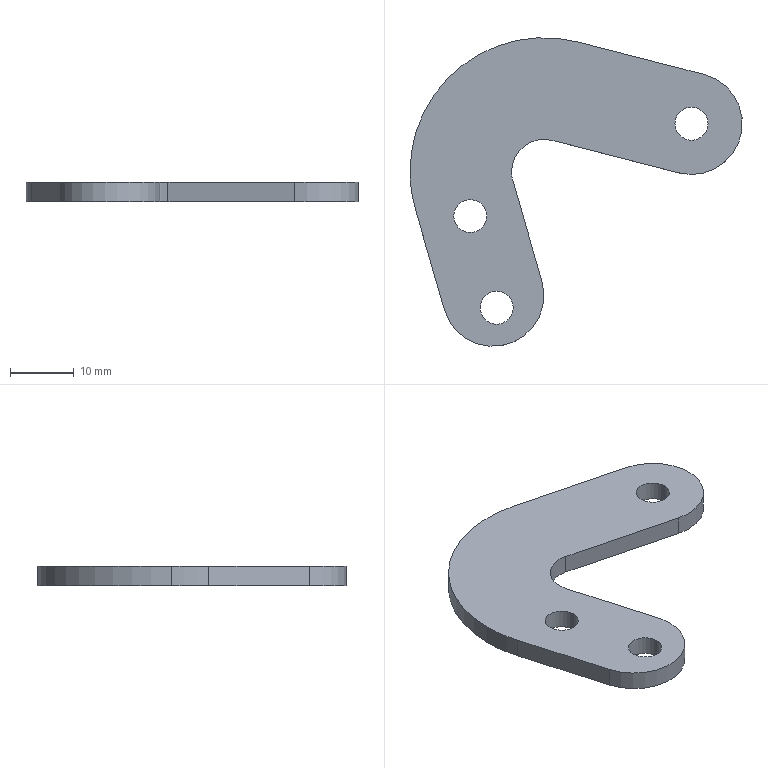Part | SolidWorks | features BaseBody 1 | 1 solid | 18 faces | box 52.312 x 48.572 x 3 mm | volume 3515 mm3 | cylinder 12 | plane 6 | commonest cylinder face diameters 5.2 x6 10.176 x2 16 x2 42.176 x2
STEP:
#1=CARTESIAN_POINT('',(-186.784,400.368,3.));
#2=VERTEX_POINT('',#1);
#3=CARTESIAN_POINT('',(-191.984,400.368,3.));
#4=VERTEX_POINT('',#3);
#5=CARTESIAN_POINT('',(-189.384,400.368,3.));
#6=DIRECTION('',(0.,0.,-1.));
#7=DIRECTION('',(-1.,0.,0.));
#8=AXIS2_PLACEMENT_3D('',#5,#6,#7);
#9=CIRCLE('',#8,2.6);
#10=EDGE_CURVE('',#2,#4,#9,.T.);
#11=ORIENTED_EDGE('',*,*,#10,.F.);
#12=CARTESIAN_POINT('',(-186.784,400.368,0.));
#13=VERTEX_POINT('',#12);
#14=CARTESIAN_POINT('',(-186.784,400.368,3.));
#15=DIRECTION('',(0.,0.,-1.));
#16=VECTOR('',#15,1000.);
#17=LINE('',#14,#16);
#18=EDGE_CURVE('',#2,#13,#17,.T.);
#19=ORIENTED_EDGE('',*,*,#18,.T.);
#20=CARTESIAN_POINT('',(-191.984,400.368,0.));
#21=VERTEX_POINT('',#20);
#22=CARTESIAN_POINT('',(-189.384,400.368,0.));
#23=DIRECTION('',(0.,0.,1.));
#24=DIRECTION('',(-1.,0.,0.));
#25=AXIS2_PLACEMENT_3D('',#22,#23,#24);
#26=CIRCLE('',#25,2.6);
#27=EDGE_CURVE('',#21,#13,#26,.T.);
#28=ORIENTED_EDGE('',*,*,#27,.F.);
#29=CARTESIAN_POINT('',(-191.984,400.368,3.));
#30=DIRECTION('',(0.,0.,-1.));
#31=VECTOR('',#30,1000.);
#32=LINE('',#29,#31);
#33=EDGE_CURVE('',#4,#21,#32,.T.);
#34=ORIENTED_EDGE('',*,*,#33,.F.);
#35=EDGE_LOOP('',(#11,#19,#28,#34));
#36=FACE_OUTER_BOUND('',#35,.T.);
#37=CARTESIAN_POINT('',(-189.384,400.368,3.));
#38=DIRECTION('',(0.,0.,-1.));
#39=DIRECTION('',(-1.,0.,0.));
#40=AXIS2_PLACEMENT_3D('',#37,#38,#39);
#41=CYLINDRICAL_SURFACE('',#40,2.6);
#42=ADVANCED_FACE('',(#36),#41,.F.);
#43=CARTESIAN_POINT('',(-198.042,401.517,3.));
#44=VERTEX_POINT('',#43);
#45=CARTESIAN_POINT('',(-198.867,407.36,3.));
#46=VERTEX_POINT('',#45);
#47=CARTESIAN_POINT('',(-177.779,407.36,3.));
#48=DIRECTION('',(0.,0.,-1.));
#49=DIRECTION('',(-1.,0.,0.));
#50=AXIS2_PLACEMENT_3D('',#47,#48,#49);
#51=CIRCLE('',#50,21.088);
#52=EDGE_CURVE('',#44,#46,#51,.T.);
#53=ORIENTED_EDGE('',*,*,#52,.T.);
#54=CARTESIAN_POINT('',(-198.867,407.36,0.));
#55=VERTEX_POINT('',#54);
#56=CARTESIAN_POINT('',(-198.867,407.36,3.));
#57=DIRECTION('',(0.,0.,-1.));
#58=VECTOR('',#57,1000.);
#59=LINE('',#56,#58);
#60=EDGE_CURVE('',#46,#55,#59,.T.);
#61=ORIENTED_EDGE('',*,*,#60,.T.);
#62=CARTESIAN_POINT('',(-198.042,401.517,0.));
#63=VERTEX_POINT('',#62);
#64=CARTESIAN_POINT('',(-177.779,407.36,0.));
#65=DIRECTION('',(0.,0.,-1.));
#66=DIRECTION('',(-1.,0.,0.));
#67=AXIS2_PLACEMENT_3D('',#64,#65,#66);
#68=CIRCLE('',#67,21.088);
#69=EDGE_CURVE('',#63,#55,#68,.T.);
#70=ORIENTED_EDGE('',*,*,#69,.F.);
#71=CARTESIAN_POINT('',(-198.042,401.517,3.));
#72=DIRECTION('',(0.,0.,1.));
#73=VECTOR('',#72,1000.);
#74=LINE('',#71,#73);
#75=EDGE_CURVE('',#63,#44,#74,.T.);
#76=ORIENTED_EDGE('',*,*,#75,.T.);
#77=EDGE_LOOP('',(#53,#61,#70,#76));
#78=FACE_OUTER_BOUND('',#77,.T.);
#79=CARTESIAN_POINT('',(-177.779,407.36,3.));
#80=DIRECTION('',(0.,0.,-1.));
#81=DIRECTION('',(-1.,0.,0.));
#82=AXIS2_PLACEMENT_3D('',#79,#80,#81);
#83=CYLINDRICAL_SURFACE('',#82,21.088);
#84=ADVANCED_FACE('',(#78),#83,.T.);
#85=CARTESIAN_POINT('',(-182.867,407.36,3.));
#86=VERTEX_POINT('',#85);
#87=CARTESIAN_POINT('',(-176.516,412.289,3.));
#88=VERTEX_POINT('',#87);
#89=CARTESIAN_POINT('',(-177.779,407.36,3.));
#90=DIRECTION('',(0.,0.,-1.));
#91=DIRECTION('',(-1.,0.,0.));
#92=AXIS2_PLACEMENT_3D('',#89,#90,#91);
#93=CIRCLE('',#92,5.088);
#94=EDGE_CURVE('',#86,#88,#93,.T.);
#95=ORIENTED_EDGE('',*,*,#94,.F.);
#96=CARTESIAN_POINT('',(-182.867,407.36,0.));
#97=VERTEX_POINT('',#96);
#98=CARTESIAN_POINT('',(-182.867,407.36,3.));
#99=DIRECTION('',(0.,0.,-1.));
#100=VECTOR('',#99,1000.);
#101=LINE('',#98,#100);
#102=EDGE_CURVE('',#86,#97,#101,.T.);
#103=ORIENTED_EDGE('',*,*,#102,.T.);
#104=CARTESIAN_POINT('',(-176.516,412.289,0.));
#105=VERTEX_POINT('',#104);
#106=CARTESIAN_POINT('',(-177.779,407.36,0.));
#107=DIRECTION('',(0.,0.,1.));
#108=DIRECTION('',(-1.,0.,0.));
#109=AXIS2_PLACEMENT_3D('',#106,#107,#108);
#110=CIRCLE('',#109,5.088);
#111=EDGE_CURVE('',#105,#97,#110,.T.);
#112=ORIENTED_EDGE('',*,*,#111,.F.);
#113=CARTESIAN_POINT('',(-176.516,412.289,3.));
#114=DIRECTION('',(0.,0.,-1.));
#115=VECTOR('',#114,1000.);
#116=LINE('',#113,#115);
#117=EDGE_CURVE('',#88,#105,#116,.T.);
#118=ORIENTED_EDGE('',*,*,#117,.F.);
#119=EDGE_LOOP('',(#95,#103,#112,#118));
#120=FACE_OUTER_BOUND('',#119,.T.);
#121=CARTESIAN_POINT('',(-177.779,407.36,3.));
#122=DIRECTION('',(0.,0.,-1.));
#123=DIRECTION('',(-1.,0.,0.));
#124=AXIS2_PLACEMENT_3D('',#121,#122,#123);
#125=CYLINDRICAL_SURFACE('',#124,5.088);
#126=ADVANCED_FACE('',(#120),#125,.F.);
#127=CARTESIAN_POINT('',(-182.628,385.955,3.));
#128=VERTEX_POINT('',#127);
#129=CARTESIAN_POINT('',(-187.828,385.955,3.));
#130=VERTEX_POINT('',#129);
#131=CARTESIAN_POINT('',(-185.228,385.955,3.));
#132=DIRECTION('',(0.,0.,-1.));
#133=DIRECTION('',(-1.,0.,0.));
#134=AXIS2_PLACEMENT_3D('',#131,#132,#133);
#135=CIRCLE('',#134,2.6);
#136=EDGE_CURVE('',#128,#130,#135,.T.);
#137=ORIENTED_EDGE('',*,*,#136,.F.);
#138=CARTESIAN_POINT('',(-182.628,385.955,0.));
#139=VERTEX_POINT('',#138);
#140=CARTESIAN_POINT('',(-182.628,385.955,3.));
#141=DIRECTION('',(0.,0.,-1.));
#142=VECTOR('',#141,1000.);
#143=LINE('',#140,#142);
#144=EDGE_CURVE('',#128,#139,#143,.T.);
#145=ORIENTED_EDGE('',*,*,#144,.T.);
#146=CARTESIAN_POINT('',(-187.828,385.955,0.));
#147=VERTEX_POINT('',#146);
#148=CARTESIAN_POINT('',(-185.228,385.955,0.));
#149=DIRECTION('',(0.,0.,1.));
#150=DIRECTION('',(-1.,0.,0.));
#151=AXIS2_PLACEMENT_3D('',#148,#149,#150);
#152=CIRCLE('',#151,2.6);
#153=EDGE_CURVE('',#147,#139,#152,.T.);
#154=ORIENTED_EDGE('',*,*,#153,.F.);
#155=CARTESIAN_POINT('',(-187.828,385.955,3.));
#156=DIRECTION('',(0.,0.,-1.));
#157=VECTOR('',#156,1000.);
#158=LINE('',#155,#157);
#159=EDGE_CURVE('',#130,#147,#158,.T.);
#160=ORIENTED_EDGE('',*,*,#159,.F.);
#161=EDGE_LOOP('',(#137,#145,#154,#160));
#162=FACE_OUTER_BOUND('',#161,.T.);
#163=CARTESIAN_POINT('',(-185.228,385.955,3.));
#164=DIRECTION('',(0.,0.,-1.));
#165=DIRECTION('',(-1.,0.,0.));
#166=AXIS2_PLACEMENT_3D('',#163,#164,#165);
#167=CYLINDRICAL_SURFACE('',#166,2.6);
#168=ADVANCED_FACE('',(#162),#167,.F.);
#169=CARTESIAN_POINT('',(-151.955,414.92,3.));
#170=VERTEX_POINT('',#169);
#171=CARTESIAN_POINT('',(-157.155,414.92,3.));
#172=VERTEX_POINT('',#171);
#173=CARTESIAN_POINT('',(-154.555,414.92,3.));
#174=DIRECTION('',(0.,0.,-1.));
#175=DIRECTION('',(-1.,0.,0.));
#176=AXIS2_PLACEMENT_3D('',#173,#174,#175);
#177=CIRCLE('',#176,2.6);
#178=EDGE_CURVE('',#170,#172,#177,.T.);
#179=ORIENTED_EDGE('',*,*,#178,.F.);
#180=CARTESIAN_POINT('',(-151.955,414.92,0.));
#181=VERTEX_POINT('',#180);
#182=CARTESIAN_POINT('',(-151.955,414.92,3.));
#183=DIRECTION('',(0.,0.,-1.));
#184=VECTOR('',#183,1000.);
#185=LINE('',#182,#184);
#186=EDGE_CURVE('',#170,#181,#185,.T.);
#187=ORIENTED_EDGE('',*,*,#186,.T.);
#188=CARTESIAN_POINT('',(-157.155,414.92,0.));
#189=VERTEX_POINT('',#188);
#190=CARTESIAN_POINT('',(-154.555,414.92,0.));
#191=DIRECTION('',(0.,0.,1.));
#192=DIRECTION('',(-1.,0.,0.));
#193=AXIS2_PLACEMENT_3D('',#190,#191,#192);
#194=CIRCLE('',#193,2.6);
#195=EDGE_CURVE('',#189,#181,#194,.T.);
#196=ORIENTED_EDGE('',*,*,#195,.F.);
#197=CARTESIAN_POINT('',(-157.155,414.92,3.));
#198=DIRECTION('',(0.,0.,-1.));
#199=VECTOR('',#198,1000.);
#200=LINE('',#197,#199);
#201=EDGE_CURVE('',#172,#189,#200,.T.);
#202=ORIENTED_EDGE('',*,*,#201,.F.);
#203=EDGE_LOOP('',(#179,#187,#196,#202));
#204=FACE_OUTER_BOUND('',#203,.T.);
#205=CARTESIAN_POINT('',(-154.555,414.92,3.));
#206=DIRECTION('',(0.,0.,-1.));
#207=DIRECTION('',(-1.,0.,0.));
#208=AXIS2_PLACEMENT_3D('',#205,#206,#207);
#209=CYLINDRICAL_SURFACE('',#208,2.6);
#210=ADVANCED_FACE('',(#204),#209,.F.);
#211=ORIENTED_EDGE('',*,*,#27,.T.);
#212=CARTESIAN_POINT('',(-189.384,400.368,0.));
#213=DIRECTION('',(0.,0.,1.));
#214=DIRECTION('',(-1.,0.,0.));
#215=AXIS2_PLACEMENT_3D('',#212,#213,#214);
#216=CIRCLE('',#215,2.6);
#217=EDGE_CURVE('',#13,#21,#216,.T.);
#218=ORIENTED_EDGE('',*,*,#217,.T.);
#219=EDGE_LOOP('',(#211,#218));
#220=FACE_BOUND('',#219,.T.);
#221=CARTESIAN_POINT('',(-172.544,427.788,0.));
#222=VERTEX_POINT('',#221);
#223=CARTESIAN_POINT('',(-152.57,422.67,0.));
#224=VERTEX_POINT('',#223);
#225=CARTESIAN_POINT('',(-172.544,427.788,0.));
#226=DIRECTION('',(0.9687,-0.2482,0.));
#227=VECTOR('',#226,1000.);
#228=LINE('',#225,#227);
#229=EDGE_CURVE('',#222,#224,#228,.T.);
#230=ORIENTED_EDGE('',*,*,#229,.T.);
#231=CARTESIAN_POINT('',(-156.541,407.171,0.));
#232=VERTEX_POINT('',#231);
#233=CARTESIAN_POINT('',(-154.555,414.92,0.));
#234=DIRECTION('',(0.,0.,-1.));
#235=DIRECTION('',(-1.,0.,0.));
#236=AXIS2_PLACEMENT_3D('',#233,#234,#235);
#237=CIRCLE('',#236,8.);
#238=EDGE_CURVE('',#224,#232,#237,.T.);
#239=ORIENTED_EDGE('',*,*,#238,.T.);
#240=CARTESIAN_POINT('',(-156.541,407.171,0.));
#241=DIRECTION('',(-0.9687,0.2482,0.));
#242=VECTOR('',#241,1000.);
#243=LINE('',#240,#242);
#244=EDGE_CURVE('',#232,#105,#243,.T.);
#245=ORIENTED_EDGE('',*,*,#244,.T.);
#246=ORIENTED_EDGE('',*,*,#111,.T.);
#247=CARTESIAN_POINT('',(-182.668,405.95,0.));
#248=VERTEX_POINT('',#247);
#249=CARTESIAN_POINT('',(-177.779,407.36,0.));
#250=DIRECTION('',(0.,0.,1.));
#251=DIRECTION('',(-1.,0.,0.));
#252=AXIS2_PLACEMENT_3D('',#249,#250,#251);
#253=CIRCLE('',#252,5.088);
#254=EDGE_CURVE('',#97,#248,#253,.T.);
#255=ORIENTED_EDGE('',*,*,#254,.T.);
#256=CARTESIAN_POINT('',(-178.095,390.093,0.));
#257=VERTEX_POINT('',#256);
#258=CARTESIAN_POINT('',(-182.668,405.95,0.));
#259=DIRECTION('',(0.2771,-0.9608,0.));
#260=VECTOR('',#259,1000.);
#261=LINE('',#258,#260);
#262=EDGE_CURVE('',#248,#257,#261,.T.);
#263=ORIENTED_EDGE('',*,*,#262,.T.);
#264=CARTESIAN_POINT('',(-193.469,385.66,0.));
#265=VERTEX_POINT('',#264);
#266=CARTESIAN_POINT('',(-185.782,387.877,0.));
#267=DIRECTION('',(0.,0.,-1.));
#268=DIRECTION('',(-1.,0.,0.));
#269=AXIS2_PLACEMENT_3D('',#266,#267,#268);
#270=CIRCLE('',#269,8.);
#271=EDGE_CURVE('',#257,#265,#270,.T.);
#272=ORIENTED_EDGE('',*,*,#271,.T.);
#273=CARTESIAN_POINT('',(-193.469,385.66,0.));
#274=DIRECTION('',(-0.2771,0.9608,0.));
#275=VECTOR('',#274,1000.);
#276=LINE('',#273,#275);
#277=EDGE_CURVE('',#265,#63,#276,.T.);
#278=ORIENTED_EDGE('',*,*,#277,.T.);
#279=ORIENTED_EDGE('',*,*,#69,.T.);
#280=CARTESIAN_POINT('',(-177.779,407.36,0.));
#281=DIRECTION('',(0.,0.,-1.));
#282=DIRECTION('',(-1.,0.,0.));
#283=AXIS2_PLACEMENT_3D('',#280,#281,#282);
#284=CIRCLE('',#283,21.088);
#285=EDGE_CURVE('',#55,#222,#284,.T.);
#286=ORIENTED_EDGE('',*,*,#285,.T.);
#287=EDGE_LOOP('',(#230,#239,#245,#246,#255,#263,#272,#278,#279,#286));
#288=FACE_OUTER_BOUND('',#287,.T.);
#289=ORIENTED_EDGE('',*,*,#153,.T.);
#290=CARTESIAN_POINT('',(-185.228,385.955,0.));
#291=DIRECTION('',(0.,0.,1.));
#292=DIRECTION('',(-1.,0.,0.));
#293=AXIS2_PLACEMENT_3D('',#290,#291,#292);
#294=CIRCLE('',#293,2.6);
#295=EDGE_CURVE('',#139,#147,#294,.T.);
#296=ORIENTED_EDGE('',*,*,#295,.T.);
#297=EDGE_LOOP('',(#289,#296));
#298=FACE_BOUND('',#297,.T.);
#299=ORIENTED_EDGE('',*,*,#195,.T.);
#300=CARTESIAN_POINT('',(-154.555,414.92,0.));
#301=DIRECTION('',(0.,0.,1.));
#302=DIRECTION('',(-1.,0.,0.));
#303=AXIS2_PLACEMENT_3D('',#300,#301,#302);
#304=CIRCLE('',#303,2.6);
#305=EDGE_CURVE('',#181,#189,#304,.T.);
#306=ORIENTED_EDGE('',*,*,#305,.T.);
#307=EDGE_LOOP('',(#299,#306));
#308=FACE_BOUND('',#307,.T.);
#309=CARTESIAN_POINT('',(-177.779,407.36,0.));
#310=DIRECTION('',(0.,0.,-1.));
#311=DIRECTION('',(-1.,0.,0.));
#312=AXIS2_PLACEMENT_3D('',#309,#310,#311);
#313=PLANE('',#312);
#314=ADVANCED_FACE('',(#220,#288,#298,#308),#313,.T.);
#315=ORIENTED_EDGE('',*,*,#18,.F.);
#316=CARTESIAN_POINT('',(-189.384,400.368,3.));
#317=DIRECTION('',(0.,0.,-1.));
#318=DIRECTION('',(-1.,0.,0.));
#319=AXIS2_PLACEMENT_3D('',#316,#317,#318);
#320=CIRCLE('',#319,2.6);
#321=EDGE_CURVE('',#4,#2,#320,.T.);
#322=ORIENTED_EDGE('',*,*,#321,.F.);
#323=ORIENTED_EDGE('',*,*,#33,.T.);
#324=ORIENTED_EDGE('',*,*,#217,.F.);
#325=EDGE_LOOP('',(#315,#322,#323,#324));
#326=FACE_OUTER_BOUND('',#325,.T.);
#327=CARTESIAN_POINT('',(-189.384,400.368,3.));
#328=DIRECTION('',(0.,0.,-1.));
#329=DIRECTION('',(-1.,0.,0.));
#330=AXIS2_PLACEMENT_3D('',#327,#328,#329);
#331=CYLINDRICAL_SURFACE('',#330,2.6);
#332=ADVANCED_FACE('',(#326),#331,.F.);
#333=ORIENTED_EDGE('',*,*,#238,.F.);
#334=CARTESIAN_POINT('',(-152.57,422.67,3.));
#335=VERTEX_POINT('',#334);
#336=CARTESIAN_POINT('',(-152.57,422.67,3.));
#337=DIRECTION('',(0.,0.,1.));
#338=VECTOR('',#337,1000.);
#339=LINE('',#336,#338);
#340=EDGE_CURVE('',#224,#335,#339,.T.);
#341=ORIENTED_EDGE('',*,*,#340,.T.);
#342=CARTESIAN_POINT('',(-156.541,407.171,3.));
#343=VERTEX_POINT('',#342);
#344=CARTESIAN_POINT('',(-154.555,414.92,3.));
#345=DIRECTION('',(0.,0.,-1.));
#346=DIRECTION('',(-1.,0.,0.));
#347=AXIS2_PLACEMENT_3D('',#344,#345,#346);
#348=CIRCLE('',#347,8.);
#349=EDGE_CURVE('',#335,#343,#348,.T.);
#350=ORIENTED_EDGE('',*,*,#349,.T.);
#351=CARTESIAN_POINT('',(-156.541,407.171,3.));
#352=DIRECTION('',(0.,0.,-1.));
#353=VECTOR('',#352,1000.);
#354=LINE('',#351,#353);
#355=EDGE_CURVE('',#343,#232,#354,.T.);
#356=ORIENTED_EDGE('',*,*,#355,.T.);
#357=EDGE_LOOP('',(#333,#341,#350,#356));
#358=FACE_OUTER_BOUND('',#357,.T.);
#359=CARTESIAN_POINT('',(-154.555,414.92,3.));
#360=DIRECTION('',(0.,0.,-1.));
#361=DIRECTION('',(-1.,0.,0.));
#362=AXIS2_PLACEMENT_3D('',#359,#360,#361);
#363=CYLINDRICAL_SURFACE('',#362,8.);
#364=ADVANCED_FACE('',(#358),#363,.T.);
#365=CARTESIAN_POINT('',(-172.544,427.788,3.));
#366=VERTEX_POINT('',#365);
#367=CARTESIAN_POINT('',(-152.57,422.67,3.));
#368=DIRECTION('',(-0.9687,0.2482,0.));
#369=VECTOR('',#368,1000.);
#370=LINE('',#367,#369);
#371=EDGE_CURVE('',#335,#366,#370,.T.);
#372=ORIENTED_EDGE('',*,*,#371,.F.);
#373=ORIENTED_EDGE('',*,*,#340,.F.);
#374=ORIENTED_EDGE('',*,*,#229,.F.);
#375=CARTESIAN_POINT('',(-172.544,427.788,3.));
#376=DIRECTION('',(0.,0.,-1.));
#377=VECTOR('',#376,1000.);
#378=LINE('',#375,#377);
#379=EDGE_CURVE('',#366,#222,#378,.T.);
#380=ORIENTED_EDGE('',*,*,#379,.F.);
#381=EDGE_LOOP('',(#372,#373,#374,#380));
#382=FACE_OUTER_BOUND('',#381,.T.);
#383=CARTESIAN_POINT('',(-152.57,422.67,3.));
#384=DIRECTION('',(-0.2482,-0.9687,0.));
#385=DIRECTION('',(0.9687,-0.2482,0.));
#386=AXIS2_PLACEMENT_3D('',#383,#384,#385);
#387=PLANE('',#386);
#388=ADVANCED_FACE('',(#382),#387,.F.);
#389=ORIENTED_EDGE('',*,*,#60,.F.);
#390=CARTESIAN_POINT('',(-177.779,407.36,3.));
#391=DIRECTION('',(0.,0.,-1.));
#392=DIRECTION('',(-1.,0.,0.));
#393=AXIS2_PLACEMENT_3D('',#390,#391,#392);
#394=CIRCLE('',#393,21.088);
#395=EDGE_CURVE('',#46,#366,#394,.T.);
#396=ORIENTED_EDGE('',*,*,#395,.T.);
#397=ORIENTED_EDGE('',*,*,#379,.T.);
#398=ORIENTED_EDGE('',*,*,#285,.F.);
#399=EDGE_LOOP('',(#389,#396,#397,#398));
#400=FACE_OUTER_BOUND('',#399,.T.);
#401=CARTESIAN_POINT('',(-177.779,407.36,3.));
#402=DIRECTION('',(0.,0.,-1.));
#403=DIRECTION('',(-1.,0.,0.));
#404=AXIS2_PLACEMENT_3D('',#401,#402,#403);
#405=CYLINDRICAL_SURFACE('',#404,21.088);
#406=ADVANCED_FACE('',(#400),#405,.T.);
#407=CARTESIAN_POINT('',(-193.469,385.66,3.));
#408=VERTEX_POINT('',#407);
#409=CARTESIAN_POINT('',(-198.042,401.517,3.));
#410=DIRECTION('',(0.2771,-0.9608,0.));
#411=VECTOR('',#410,1000.);
#412=LINE('',#409,#411);
#413=EDGE_CURVE('',#44,#408,#412,.T.);
#414=ORIENTED_EDGE('',*,*,#413,.F.);
#415=ORIENTED_EDGE('',*,*,#75,.F.);
#416=ORIENTED_EDGE('',*,*,#277,.F.);
#417=CARTESIAN_POINT('',(-193.469,385.66,3.));
#418=DIRECTION('',(0.,0.,-1.));
#419=VECTOR('',#418,1000.);
#420=LINE('',#417,#419);
#421=EDGE_CURVE('',#408,#265,#420,.T.);
#422=ORIENTED_EDGE('',*,*,#421,.F.);
#423=EDGE_LOOP('',(#414,#415,#416,#422));
#424=FACE_OUTER_BOUND('',#423,.T.);
#425=CARTESIAN_POINT('',(-198.042,401.517,3.));
#426=DIRECTION('',(0.9608,0.2771,0.));
#427=DIRECTION('',(-0.2771,0.9608,0.));
#428=AXIS2_PLACEMENT_3D('',#425,#426,#427);
#429=PLANE('',#428);
#430=ADVANCED_FACE('',(#424),#429,.F.);
#431=ORIENTED_EDGE('',*,*,#271,.F.);
#432=CARTESIAN_POINT('',(-178.095,390.093,3.));
#433=VERTEX_POINT('',#432);
#434=CARTESIAN_POINT('',(-178.095,390.093,3.));
#435=DIRECTION('',(0.,0.,1.));
#436=VECTOR('',#435,1000.);
#437=LINE('',#434,#436);
#438=EDGE_CURVE('',#257,#433,#437,.T.);
#439=ORIENTED_EDGE('',*,*,#438,.T.);
#440=CARTESIAN_POINT('',(-185.782,387.877,3.));
#441=DIRECTION('',(0.,0.,-1.));
#442=DIRECTION('',(-1.,0.,0.));
#443=AXIS2_PLACEMENT_3D('',#440,#441,#442);
#444=CIRCLE('',#443,8.);
#445=EDGE_CURVE('',#433,#408,#444,.T.);
#446=ORIENTED_EDGE('',*,*,#445,.T.);
#447=ORIENTED_EDGE('',*,*,#421,.T.);
#448=EDGE_LOOP('',(#431,#439,#446,#447));
#449=FACE_OUTER_BOUND('',#448,.T.);
#450=CARTESIAN_POINT('',(-185.782,387.877,3.));
#451=DIRECTION('',(0.,0.,-1.));
#452=DIRECTION('',(-1.,0.,0.));
#453=AXIS2_PLACEMENT_3D('',#450,#451,#452);
#454=CYLINDRICAL_SURFACE('',#453,8.);
#455=ADVANCED_FACE('',(#449),#454,.T.);
#456=CARTESIAN_POINT('',(-182.668,405.95,3.));
#457=VERTEX_POINT('',#456);
#458=CARTESIAN_POINT('',(-178.095,390.093,3.));
#459=DIRECTION('',(-0.2771,0.9608,0.));
#460=VECTOR('',#459,1000.);
#461=LINE('',#458,#460);
#462=EDGE_CURVE('',#433,#457,#461,.T.);
#463=ORIENTED_EDGE('',*,*,#462,.F.);
#464=ORIENTED_EDGE('',*,*,#438,.F.);
#465=ORIENTED_EDGE('',*,*,#262,.F.);
#466=CARTESIAN_POINT('',(-182.668,405.95,3.));
#467=DIRECTION('',(0.,0.,-1.));
#468=VECTOR('',#467,1000.);
#469=LINE('',#466,#468);
#470=EDGE_CURVE('',#457,#248,#469,.T.);
#471=ORIENTED_EDGE('',*,*,#470,.F.);
#472=EDGE_LOOP('',(#463,#464,#465,#471));
#473=FACE_OUTER_BOUND('',#472,.T.);
#474=CARTESIAN_POINT('',(-178.095,390.093,3.));
#475=DIRECTION('',(-0.9608,-0.2771,0.));
#476=DIRECTION('',(0.2771,-0.9608,0.));
#477=AXIS2_PLACEMENT_3D('',#474,#475,#476);
#478=PLANE('',#477);
#479=ADVANCED_FACE('',(#473),#478,.F.);
#480=ORIENTED_EDGE('',*,*,#102,.F.);
#481=CARTESIAN_POINT('',(-177.779,407.36,3.));
#482=DIRECTION('',(0.,0.,-1.));
#483=DIRECTION('',(-1.,0.,0.));
#484=AXIS2_PLACEMENT_3D('',#481,#482,#483);
#485=CIRCLE('',#484,5.088);
#486=EDGE_CURVE('',#457,#86,#485,.T.);
#487=ORIENTED_EDGE('',*,*,#486,.F.);
#488=ORIENTED_EDGE('',*,*,#470,.T.);
#489=ORIENTED_EDGE('',*,*,#254,.F.);
#490=EDGE_LOOP('',(#480,#487,#488,#489));
#491=FACE_OUTER_BOUND('',#490,.T.);
#492=CARTESIAN_POINT('',(-177.779,407.36,3.));
#493=DIRECTION('',(0.,0.,-1.));
#494=DIRECTION('',(-1.,0.,0.));
#495=AXIS2_PLACEMENT_3D('',#492,#493,#494);
#496=CYLINDRICAL_SURFACE('',#495,5.088);
#497=ADVANCED_FACE('',(#491),#496,.F.);
#498=CARTESIAN_POINT('',(-176.516,412.289,3.));
#499=DIRECTION('',(0.9687,-0.2482,0.));
#500=VECTOR('',#499,1000.);
#501=LINE('',#498,#500);
#502=EDGE_CURVE('',#88,#343,#501,.T.);
#503=ORIENTED_EDGE('',*,*,#502,.F.);
#504=ORIENTED_EDGE('',*,*,#117,.T.);
#505=ORIENTED_EDGE('',*,*,#244,.F.);
#506=ORIENTED_EDGE('',*,*,#355,.F.);
#507=EDGE_LOOP('',(#503,#504,#505,#506));
#508=FACE_OUTER_BOUND('',#507,.T.);
#509=CARTESIAN_POINT('',(-176.516,412.289,3.));
#510=DIRECTION('',(0.2482,0.9687,0.));
#511=DIRECTION('',(-0.9687,0.2482,0.));
#512=AXIS2_PLACEMENT_3D('',#509,#510,#511);
#513=PLANE('',#512);
#514=ADVANCED_FACE('',(#508),#513,.F.);
#515=ORIENTED_EDGE('',*,*,#144,.F.);
#516=CARTESIAN_POINT('',(-185.228,385.955,3.));
#517=DIRECTION('',(0.,0.,-1.));
#518=DIRECTION('',(-1.,0.,0.));
#519=AXIS2_PLACEMENT_3D('',#516,#517,#518);
#520=CIRCLE('',#519,2.6);
#521=EDGE_CURVE('',#130,#128,#520,.T.);
#522=ORIENTED_EDGE('',*,*,#521,.F.);
#523=ORIENTED_EDGE('',*,*,#159,.T.);
#524=ORIENTED_EDGE('',*,*,#295,.F.);
#525=EDGE_LOOP('',(#515,#522,#523,#524));
#526=FACE_OUTER_BOUND('',#525,.T.);
#527=CARTESIAN_POINT('',(-185.228,385.955,3.));
#528=DIRECTION('',(0.,0.,-1.));
#529=DIRECTION('',(-1.,0.,0.));
#530=AXIS2_PLACEMENT_3D('',#527,#528,#529);
#531=CYLINDRICAL_SURFACE('',#530,2.6);
#532=ADVANCED_FACE('',(#526),#531,.F.);
#533=ORIENTED_EDGE('',*,*,#186,.F.);
#534=CARTESIAN_POINT('',(-154.555,414.92,3.));
#535=DIRECTION('',(0.,0.,-1.));
#536=DIRECTION('',(-1.,0.,0.));
#537=AXIS2_PLACEMENT_3D('',#534,#535,#536);
#538=CIRCLE('',#537,2.6);
#539=EDGE_CURVE('',#172,#170,#538,.T.);
#540=ORIENTED_EDGE('',*,*,#539,.F.);
#541=ORIENTED_EDGE('',*,*,#201,.T.);
#542=ORIENTED_EDGE('',*,*,#305,.F.);
#543=EDGE_LOOP('',(#533,#540,#541,#542));
#544=FACE_OUTER_BOUND('',#543,.T.);
#545=CARTESIAN_POINT('',(-154.555,414.92,3.));
#546=DIRECTION('',(0.,0.,-1.));
#547=DIRECTION('',(-1.,0.,0.));
#548=AXIS2_PLACEMENT_3D('',#545,#546,#547);
#549=CYLINDRICAL_SURFACE('',#548,2.6);
#550=ADVANCED_FACE('',(#544),#549,.F.);
#551=ORIENTED_EDGE('',*,*,#486,.T.);
#552=ORIENTED_EDGE('',*,*,#94,.T.);
#553=ORIENTED_EDGE('',*,*,#502,.T.);
#554=ORIENTED_EDGE('',*,*,#349,.F.);
#555=ORIENTED_EDGE('',*,*,#371,.T.);
#556=ORIENTED_EDGE('',*,*,#395,.F.);
#557=ORIENTED_EDGE('',*,*,#52,.F.);
#558=ORIENTED_EDGE('',*,*,#413,.T.);
#559=ORIENTED_EDGE('',*,*,#445,.F.);
#560=ORIENTED_EDGE('',*,*,#462,.T.);
#561=EDGE_LOOP('',(#551,#552,#553,#554,#555,#556,#557,#558,#559,#560));
#562=FACE_OUTER_BOUND('',#561,.T.);
#563=ORIENTED_EDGE('',*,*,#521,.T.);
#564=ORIENTED_EDGE('',*,*,#136,.T.);
#565=EDGE_LOOP('',(#563,#564));
#566=FACE_BOUND('',#565,.T.);
#567=ORIENTED_EDGE('',*,*,#321,.T.);
#568=ORIENTED_EDGE('',*,*,#10,.T.);
#569=EDGE_LOOP('',(#567,#568));
#570=FACE_BOUND('',#569,.T.);
#571=ORIENTED_EDGE('',*,*,#539,.T.);
#572=ORIENTED_EDGE('',*,*,#178,.T.);
#573=EDGE_LOOP('',(#571,#572));
#574=FACE_BOUND('',#573,.T.);
#575=CARTESIAN_POINT('',(-177.779,407.36,3.));
#576=DIRECTION('',(0.,0.,-1.));
#577=DIRECTION('',(-1.,0.,0.));
#578=AXIS2_PLACEMENT_3D('',#575,#576,#577);
#579=PLANE('',#578);
#580=ADVANCED_FACE('',(#562,#566,#570,#574),#579,.F.);
#581=CLOSED_SHELL('',(#42,#84,#126,#168,#210,#314,#332,#364,#388,#406,#430,#455,#479,#497,#514,#532,#550,#580));
#582=MANIFOLD_SOLID_BREP('',#581);
#583=CARTESIAN_POINT('',(0.,0.,0.));
#584=DIRECTION('',(0.,0.,1.));
#585=DIRECTION('',(1.,0.,0.));
#586=AXIS2_PLACEMENT_3D('',#583,#584,#585);
#587=(LENGTH_UNIT()NAMED_UNIT(*)SI_UNIT(.MILLI.,.METRE.));
#588=UNCERTAINTY_MEASURE_WITH_UNIT(LENGTH_MEASURE(0.00001),#587,'','');
#589=(NAMED_UNIT(*)PLANE_ANGLE_UNIT()SI_UNIT($,.RADIAN.));
#590=(NAMED_UNIT(*)SI_UNIT($,.STERADIAN.)SOLID_ANGLE_UNIT());
#591=(GEOMETRIC_REPRESENTATION_CONTEXT(3)GLOBAL_UNCERTAINTY_ASSIGNED_CONTEXT((#588))GLOBAL_UNIT_ASSIGNED_CONTEXT((#587,#589,#590))REPRESENTATION_CONTEXT('',''));
#592=ADVANCED_BREP_SHAPE_REPRESENTATION('',(#582,#586),#591);